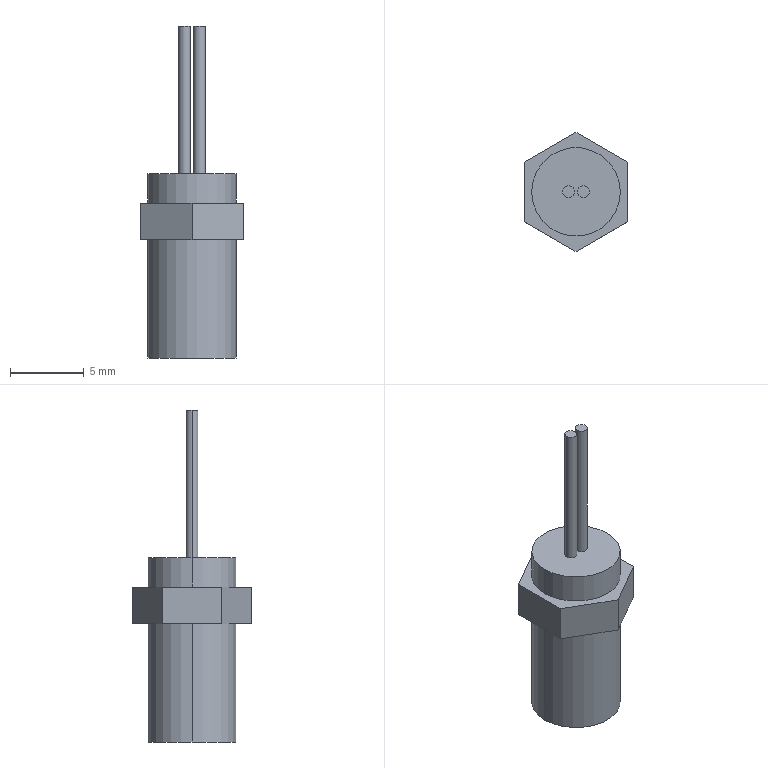Part | SolidWorks | features ICE 3, Extrusion 1 | 1 solid | 20 faces | box 7 x 8.083 x 22.5 mm | volume 398.885 mm3 | plane 12 | cylinder 8 | commonest cylinder face diameters 0.8 x4 6 x4
STEP:
#1=CARTESIAN_POINT('',(-0.1,0.,22.5));
#2=VERTEX_POINT('',#1);
#3=CARTESIAN_POINT('',(-0.9,0.,22.5));
#4=VERTEX_POINT('',#3);
#5=CARTESIAN_POINT('',(-0.5,0.,22.5));
#6=DIRECTION('',(0.,0.,1.));
#7=DIRECTION('',(1.,0.,0.));
#8=AXIS2_PLACEMENT_3D('',#5,#6,#7);
#9=CIRCLE('',#8,0.4);
#10=EDGE_CURVE('',#2,#4,#9,.T.);
#11=ORIENTED_EDGE('',*,*,#10,.F.);
#12=CARTESIAN_POINT('',(-0.1,0.,12.5));
#13=VERTEX_POINT('',#12);
#14=CARTESIAN_POINT('',(-0.1,0.,22.5));
#15=DIRECTION('',(0.,0.,-1.));
#16=VECTOR('',#15,1000.);
#17=LINE('',#14,#16);
#18=EDGE_CURVE('',#2,#13,#17,.T.);
#19=ORIENTED_EDGE('',*,*,#18,.T.);
#20=CARTESIAN_POINT('',(-0.9,0.,12.5));
#21=VERTEX_POINT('',#20);
#22=CARTESIAN_POINT('',(-0.5,0.,12.5));
#23=DIRECTION('',(0.,0.,1.));
#24=DIRECTION('',(1.,0.,0.));
#25=AXIS2_PLACEMENT_3D('',#22,#23,#24);
#26=CIRCLE('',#25,0.4);
#27=EDGE_CURVE('',#13,#21,#26,.T.);
#28=ORIENTED_EDGE('',*,*,#27,.T.);
#29=CARTESIAN_POINT('',(-0.9,0.,22.5));
#30=DIRECTION('',(0.,0.,-1.));
#31=VECTOR('',#30,1000.);
#32=LINE('',#29,#31);
#33=EDGE_CURVE('',#4,#21,#32,.T.);
#34=ORIENTED_EDGE('',*,*,#33,.F.);
#35=EDGE_LOOP('',(#11,#19,#28,#34));
#36=FACE_OUTER_BOUND('',#35,.T.);
#37=CARTESIAN_POINT('',(-0.5,0.,22.5));
#38=DIRECTION('',(0.,0.,-1.));
#39=DIRECTION('',(-1.,0.,0.));
#40=AXIS2_PLACEMENT_3D('',#37,#38,#39);
#41=CYLINDRICAL_SURFACE('',#40,0.4);
#42=ADVANCED_FACE('',(#36),#41,.T.);
#43=CARTESIAN_POINT('',(0.9,0.,22.5));
#44=VERTEX_POINT('',#43);
#45=CARTESIAN_POINT('',(0.1,0.,22.5));
#46=VERTEX_POINT('',#45);
#47=CARTESIAN_POINT('',(0.5,0.,22.5));
#48=DIRECTION('',(0.,0.,1.));
#49=DIRECTION('',(1.,0.,0.));
#50=AXIS2_PLACEMENT_3D('',#47,#48,#49);
#51=CIRCLE('',#50,0.4);
#52=EDGE_CURVE('',#44,#46,#51,.T.);
#53=ORIENTED_EDGE('',*,*,#52,.F.);
#54=CARTESIAN_POINT('',(0.9,0.,12.5));
#55=VERTEX_POINT('',#54);
#56=CARTESIAN_POINT('',(0.9,0.,22.5));
#57=DIRECTION('',(0.,0.,-1.));
#58=VECTOR('',#57,1000.);
#59=LINE('',#56,#58);
#60=EDGE_CURVE('',#44,#55,#59,.T.);
#61=ORIENTED_EDGE('',*,*,#60,.T.);
#62=CARTESIAN_POINT('',(0.1,0.,12.5));
#63=VERTEX_POINT('',#62);
#64=CARTESIAN_POINT('',(0.5,0.,12.5));
#65=DIRECTION('',(0.,0.,1.));
#66=DIRECTION('',(1.,0.,0.));
#67=AXIS2_PLACEMENT_3D('',#64,#65,#66);
#68=CIRCLE('',#67,0.4);
#69=EDGE_CURVE('',#55,#63,#68,.T.);
#70=ORIENTED_EDGE('',*,*,#69,.T.);
#71=CARTESIAN_POINT('',(0.1,0.,22.5));
#72=DIRECTION('',(0.,0.,-1.));
#73=VECTOR('',#72,1000.);
#74=LINE('',#71,#73);
#75=EDGE_CURVE('',#46,#63,#74,.T.);
#76=ORIENTED_EDGE('',*,*,#75,.F.);
#77=EDGE_LOOP('',(#53,#61,#70,#76));
#78=FACE_OUTER_BOUND('',#77,.T.);
#79=CARTESIAN_POINT('',(0.5,0.,22.5));
#80=DIRECTION('',(0.,0.,-1.));
#81=DIRECTION('',(-1.,0.,0.));
#82=AXIS2_PLACEMENT_3D('',#79,#80,#81);
#83=CYLINDRICAL_SURFACE('',#82,0.4);
#84=ADVANCED_FACE('',(#78),#83,.T.);
#85=CARTESIAN_POINT('',(3.,0.,12.5));
#86=VERTEX_POINT('',#85);
#87=CARTESIAN_POINT('',(-3.,0.,12.5));
#88=VERTEX_POINT('',#87);
#89=CARTESIAN_POINT('',(0.,0.,12.5));
#90=DIRECTION('',(0.,0.,1.));
#91=DIRECTION('',(1.,0.,0.));
#92=AXIS2_PLACEMENT_3D('',#89,#90,#91);
#93=CIRCLE('',#92,3.);
#94=EDGE_CURVE('',#86,#88,#93,.T.);
#95=ORIENTED_EDGE('',*,*,#94,.F.);
#96=CARTESIAN_POINT('',(3.,0.,10.5));
#97=VERTEX_POINT('',#96);
#98=CARTESIAN_POINT('',(3.,0.,12.5));
#99=DIRECTION('',(0.,0.,-1.));
#100=VECTOR('',#99,1000.);
#101=LINE('',#98,#100);
#102=EDGE_CURVE('',#86,#97,#101,.T.);
#103=ORIENTED_EDGE('',*,*,#102,.T.);
#104=CARTESIAN_POINT('',(-3.,0.,10.5));
#105=VERTEX_POINT('',#104);
#106=CARTESIAN_POINT('',(0.,0.,10.5));
#107=DIRECTION('',(0.,0.,1.));
#108=DIRECTION('',(1.,0.,0.));
#109=AXIS2_PLACEMENT_3D('',#106,#107,#108);
#110=CIRCLE('',#109,3.);
#111=EDGE_CURVE('',#97,#105,#110,.T.);
#112=ORIENTED_EDGE('',*,*,#111,.T.);
#113=CARTESIAN_POINT('',(-3.,0.,12.5));
#114=DIRECTION('',(0.,0.,-1.));
#115=VECTOR('',#114,1000.);
#116=LINE('',#113,#115);
#117=EDGE_CURVE('',#88,#105,#116,.T.);
#118=ORIENTED_EDGE('',*,*,#117,.F.);
#119=EDGE_LOOP('',(#95,#103,#112,#118));
#120=FACE_OUTER_BOUND('',#119,.T.);
#121=CARTESIAN_POINT('',(0.,0.,12.5));
#122=DIRECTION('',(0.,0.,-1.));
#123=DIRECTION('',(-1.,0.,0.));
#124=AXIS2_PLACEMENT_3D('',#121,#122,#123);
#125=CYLINDRICAL_SURFACE('',#124,3.);
#126=ADVANCED_FACE('',(#120),#125,.T.);
#127=CARTESIAN_POINT('',(3.,0.,8.));
#128=VERTEX_POINT('',#127);
#129=CARTESIAN_POINT('',(-3.,0.,8.));
#130=VERTEX_POINT('',#129);
#131=CARTESIAN_POINT('',(0.,0.,8.));
#132=DIRECTION('',(0.,0.,1.));
#133=DIRECTION('',(1.,0.,0.));
#134=AXIS2_PLACEMENT_3D('',#131,#132,#133);
#135=CIRCLE('',#134,3.);
#136=EDGE_CURVE('',#128,#130,#135,.T.);
#137=ORIENTED_EDGE('',*,*,#136,.F.);
#138=CARTESIAN_POINT('',(3.,0.,0.));
#139=VERTEX_POINT('',#138);
#140=CARTESIAN_POINT('',(3.,0.,8.));
#141=DIRECTION('',(0.,0.,-1.));
#142=VECTOR('',#141,1000.);
#143=LINE('',#140,#142);
#144=EDGE_CURVE('',#128,#139,#143,.T.);
#145=ORIENTED_EDGE('',*,*,#144,.T.);
#146=CARTESIAN_POINT('',(-3.,0.,0.));
#147=VERTEX_POINT('',#146);
#148=CARTESIAN_POINT('',(0.,0.,0.));
#149=DIRECTION('',(0.,0.,1.));
#150=DIRECTION('',(1.,0.,0.));
#151=AXIS2_PLACEMENT_3D('',#148,#149,#150);
#152=CIRCLE('',#151,3.);
#153=EDGE_CURVE('',#139,#147,#152,.T.);
#154=ORIENTED_EDGE('',*,*,#153,.T.);
#155=CARTESIAN_POINT('',(-3.,0.,8.));
#156=DIRECTION('',(0.,0.,-1.));
#157=VECTOR('',#156,1000.);
#158=LINE('',#155,#157);
#159=EDGE_CURVE('',#130,#147,#158,.T.);
#160=ORIENTED_EDGE('',*,*,#159,.F.);
#161=EDGE_LOOP('',(#137,#145,#154,#160));
#162=FACE_OUTER_BOUND('',#161,.T.);
#163=CARTESIAN_POINT('',(0.,0.,8.));
#164=DIRECTION('',(0.,0.,-1.));
#165=DIRECTION('',(-1.,0.,0.));
#166=AXIS2_PLACEMENT_3D('',#163,#164,#165);
#167=CYLINDRICAL_SURFACE('',#166,3.);
#168=ADVANCED_FACE('',(#162),#167,.T.);
#169=CARTESIAN_POINT('',(0.5,0.,12.5));
#170=DIRECTION('',(0.,0.,1.));
#171=DIRECTION('',(1.,0.,0.));
#172=AXIS2_PLACEMENT_3D('',#169,#170,#171);
#173=CIRCLE('',#172,0.4);
#174=EDGE_CURVE('',#63,#55,#173,.T.);
#175=ORIENTED_EDGE('',*,*,#174,.F.);
#176=ORIENTED_EDGE('',*,*,#69,.F.);
#177=EDGE_LOOP('',(#175,#176));
#178=FACE_BOUND('',#177,.T.);
#179=CARTESIAN_POINT('',(0.,0.,12.5));
#180=DIRECTION('',(0.,0.,1.));
#181=DIRECTION('',(1.,0.,0.));
#182=AXIS2_PLACEMENT_3D('',#179,#180,#181);
#183=CIRCLE('',#182,3.);
#184=EDGE_CURVE('',#88,#86,#183,.T.);
#185=ORIENTED_EDGE('',*,*,#184,.T.);
#186=ORIENTED_EDGE('',*,*,#94,.T.);
#187=EDGE_LOOP('',(#185,#186));
#188=FACE_OUTER_BOUND('',#187,.T.);
#189=CARTESIAN_POINT('',(-0.5,0.,12.5));
#190=DIRECTION('',(0.,0.,1.));
#191=DIRECTION('',(1.,0.,0.));
#192=AXIS2_PLACEMENT_3D('',#189,#190,#191);
#193=CIRCLE('',#192,0.4);
#194=EDGE_CURVE('',#21,#13,#193,.T.);
#195=ORIENTED_EDGE('',*,*,#194,.F.);
#196=ORIENTED_EDGE('',*,*,#27,.F.);
#197=EDGE_LOOP('',(#195,#196));
#198=FACE_BOUND('',#197,.T.);
#199=CARTESIAN_POINT('',(0.,0.,12.5));
#200=DIRECTION('',(0.,0.,1.));
#201=DIRECTION('',(1.,0.,0.));
#202=AXIS2_PLACEMENT_3D('',#199,#200,#201);
#203=PLANE('',#202);
#204=ADVANCED_FACE('',(#178,#188,#198),#203,.T.);
#205=CARTESIAN_POINT('',(3.5,2.021,10.5));
#206=VERTEX_POINT('',#205);
#207=CARTESIAN_POINT('',(0.,4.041,10.5));
#208=VERTEX_POINT('',#207);
#209=CARTESIAN_POINT('',(3.5,2.021,10.5));
#210=DIRECTION('',(-0.866,0.5,0.));
#211=VECTOR('',#210,1000.);
#212=LINE('',#209,#211);
#213=EDGE_CURVE('',#206,#208,#212,.T.);
#214=ORIENTED_EDGE('',*,*,#213,.T.);
#215=CARTESIAN_POINT('',(-3.5,2.021,10.5));
#216=VERTEX_POINT('',#215);
#217=CARTESIAN_POINT('',(0.,4.041,10.5));
#218=DIRECTION('',(-0.866,-0.5,0.));
#219=VECTOR('',#218,1000.);
#220=LINE('',#217,#219);
#221=EDGE_CURVE('',#208,#216,#220,.T.);
#222=ORIENTED_EDGE('',*,*,#221,.T.);
#223=CARTESIAN_POINT('',(-3.5,-2.021,10.5));
#224=VERTEX_POINT('',#223);
#225=CARTESIAN_POINT('',(-3.5,2.021,10.5));
#226=DIRECTION('',(0.,-1.,0.));
#227=VECTOR('',#226,1000.);
#228=LINE('',#225,#227);
#229=EDGE_CURVE('',#216,#224,#228,.T.);
#230=ORIENTED_EDGE('',*,*,#229,.T.);
#231=CARTESIAN_POINT('',(0.,-4.041,10.5));
#232=VERTEX_POINT('',#231);
#233=CARTESIAN_POINT('',(-3.5,-2.021,10.5));
#234=DIRECTION('',(0.866,-0.5,0.));
#235=VECTOR('',#234,1000.);
#236=LINE('',#233,#235);
#237=EDGE_CURVE('',#224,#232,#236,.T.);
#238=ORIENTED_EDGE('',*,*,#237,.T.);
#239=CARTESIAN_POINT('',(3.5,-2.021,10.5));
#240=VERTEX_POINT('',#239);
#241=CARTESIAN_POINT('',(0.,-4.041,10.5));
#242=DIRECTION('',(0.866,0.5,0.));
#243=VECTOR('',#242,1000.);
#244=LINE('',#241,#243);
#245=EDGE_CURVE('',#232,#240,#244,.T.);
#246=ORIENTED_EDGE('',*,*,#245,.T.);
#247=CARTESIAN_POINT('',(3.5,-2.021,10.5));
#248=DIRECTION('',(0.,1.,0.));
#249=VECTOR('',#248,1000.);
#250=LINE('',#247,#249);
#251=EDGE_CURVE('',#240,#206,#250,.T.);
#252=ORIENTED_EDGE('',*,*,#251,.T.);
#253=EDGE_LOOP('',(#214,#222,#230,#238,#246,#252));
#254=FACE_OUTER_BOUND('',#253,.T.);
#255=CARTESIAN_POINT('',(0.,0.,10.5));
#256=DIRECTION('',(0.,0.,1.));
#257=DIRECTION('',(1.,0.,0.));
#258=AXIS2_PLACEMENT_3D('',#255,#256,#257);
#259=CIRCLE('',#258,3.);
#260=EDGE_CURVE('',#105,#97,#259,.T.);
#261=ORIENTED_EDGE('',*,*,#260,.F.);
#262=ORIENTED_EDGE('',*,*,#111,.F.);
#263=EDGE_LOOP('',(#261,#262));
#264=FACE_BOUND('',#263,.T.);
#265=CARTESIAN_POINT('',(0.,0.,10.5));
#266=DIRECTION('',(0.,0.,1.));
#267=DIRECTION('',(1.,0.,0.));
#268=AXIS2_PLACEMENT_3D('',#265,#266,#267);
#269=PLANE('',#268);
#270=ADVANCED_FACE('',(#254,#264),#269,.T.);
#271=ORIENTED_EDGE('',*,*,#144,.F.);
#272=CARTESIAN_POINT('',(0.,0.,8.));
#273=DIRECTION('',(0.,0.,1.));
#274=DIRECTION('',(1.,0.,0.));
#275=AXIS2_PLACEMENT_3D('',#272,#273,#274);
#276=CIRCLE('',#275,3.);
#277=EDGE_CURVE('',#130,#128,#276,.T.);
#278=ORIENTED_EDGE('',*,*,#277,.F.);
#279=ORIENTED_EDGE('',*,*,#159,.T.);
#280=CARTESIAN_POINT('',(0.,0.,0.));
#281=DIRECTION('',(0.,0.,1.));
#282=DIRECTION('',(1.,0.,0.));
#283=AXIS2_PLACEMENT_3D('',#280,#281,#282);
#284=CIRCLE('',#283,3.);
#285=EDGE_CURVE('',#147,#139,#284,.T.);
#286=ORIENTED_EDGE('',*,*,#285,.T.);
#287=EDGE_LOOP('',(#271,#278,#279,#286));
#288=FACE_OUTER_BOUND('',#287,.T.);
#289=CARTESIAN_POINT('',(0.,0.,8.));
#290=DIRECTION('',(0.,0.,-1.));
#291=DIRECTION('',(-1.,0.,0.));
#292=AXIS2_PLACEMENT_3D('',#289,#290,#291);
#293=CYLINDRICAL_SURFACE('',#292,3.);
#294=ADVANCED_FACE('',(#288),#293,.T.);
#295=ORIENTED_EDGE('',*,*,#285,.F.);
#296=ORIENTED_EDGE('',*,*,#153,.F.);
#297=EDGE_LOOP('',(#295,#296));
#298=FACE_OUTER_BOUND('',#297,.T.);
#299=CARTESIAN_POINT('',(0.,0.,0.));
#300=DIRECTION('',(0.,0.,1.));
#301=DIRECTION('',(1.,0.,0.));
#302=AXIS2_PLACEMENT_3D('',#299,#300,#301);
#303=PLANE('',#302);
#304=ADVANCED_FACE('',(#298),#303,.F.);
#305=CARTESIAN_POINT('',(3.5,2.021,8.));
#306=VERTEX_POINT('',#305);
#307=CARTESIAN_POINT('',(0.,4.041,8.));
#308=VERTEX_POINT('',#307);
#309=CARTESIAN_POINT('',(3.5,2.021,8.));
#310=DIRECTION('',(-0.866,0.5,0.));
#311=VECTOR('',#310,1000.);
#312=LINE('',#309,#311);
#313=EDGE_CURVE('',#306,#308,#312,.T.);
#314=ORIENTED_EDGE('',*,*,#313,.F.);
#315=CARTESIAN_POINT('',(3.5,-2.021,8.));
#316=VERTEX_POINT('',#315);
#317=CARTESIAN_POINT('',(3.5,-2.021,8.));
#318=DIRECTION('',(0.,1.,0.));
#319=VECTOR('',#318,1000.);
#320=LINE('',#317,#319);
#321=EDGE_CURVE('',#316,#306,#320,.T.);
#322=ORIENTED_EDGE('',*,*,#321,.F.);
#323=CARTESIAN_POINT('',(0.,-4.041,8.));
#324=VERTEX_POINT('',#323);
#325=CARTESIAN_POINT('',(0.,-4.041,8.));
#326=DIRECTION('',(0.866,0.5,0.));
#327=VECTOR('',#326,1000.);
#328=LINE('',#325,#327);
#329=EDGE_CURVE('',#324,#316,#328,.T.);
#330=ORIENTED_EDGE('',*,*,#329,.F.);
#331=CARTESIAN_POINT('',(-3.5,-2.021,8.));
#332=VERTEX_POINT('',#331);
#333=CARTESIAN_POINT('',(-3.5,-2.021,8.));
#334=DIRECTION('',(0.866,-0.5,0.));
#335=VECTOR('',#334,1000.);
#336=LINE('',#333,#335);
#337=EDGE_CURVE('',#332,#324,#336,.T.);
#338=ORIENTED_EDGE('',*,*,#337,.F.);
#339=CARTESIAN_POINT('',(-3.5,2.021,8.));
#340=VERTEX_POINT('',#339);
#341=CARTESIAN_POINT('',(-3.5,2.021,8.));
#342=DIRECTION('',(0.,-1.,0.));
#343=VECTOR('',#342,1000.);
#344=LINE('',#341,#343);
#345=EDGE_CURVE('',#340,#332,#344,.T.);
#346=ORIENTED_EDGE('',*,*,#345,.F.);
#347=CARTESIAN_POINT('',(0.,4.041,8.));
#348=DIRECTION('',(-0.866,-0.5,0.));
#349=VECTOR('',#348,1000.);
#350=LINE('',#347,#349);
#351=EDGE_CURVE('',#308,#340,#350,.T.);
#352=ORIENTED_EDGE('',*,*,#351,.F.);
#353=EDGE_LOOP('',(#314,#322,#330,#338,#346,#352));
#354=FACE_OUTER_BOUND('',#353,.T.);
#355=ORIENTED_EDGE('',*,*,#277,.T.);
#356=ORIENTED_EDGE('',*,*,#136,.T.);
#357=EDGE_LOOP('',(#355,#356));
#358=FACE_BOUND('',#357,.T.);
#359=CARTESIAN_POINT('',(0.,0.,8.));
#360=DIRECTION('',(0.,0.,1.));
#361=DIRECTION('',(1.,0.,0.));
#362=AXIS2_PLACEMENT_3D('',#359,#360,#361);
#363=PLANE('',#362);
#364=ADVANCED_FACE('',(#354,#358),#363,.F.);
#365=ORIENTED_EDGE('',*,*,#313,.T.);
#366=CARTESIAN_POINT('',(0.,4.041,10.5));
#367=DIRECTION('',(0.,0.,-1.));
#368=VECTOR('',#367,1000.);
#369=LINE('',#366,#368);
#370=EDGE_CURVE('',#208,#308,#369,.T.);
#371=ORIENTED_EDGE('',*,*,#370,.F.);
#372=ORIENTED_EDGE('',*,*,#213,.F.);
#373=CARTESIAN_POINT('',(3.5,2.021,10.5));
#374=DIRECTION('',(0.,0.,-1.));
#375=VECTOR('',#374,1000.);
#376=LINE('',#373,#375);
#377=EDGE_CURVE('',#206,#306,#376,.T.);
#378=ORIENTED_EDGE('',*,*,#377,.T.);
#379=EDGE_LOOP('',(#365,#371,#372,#378));
#380=FACE_OUTER_BOUND('',#379,.T.);
#381=CARTESIAN_POINT('',(3.5,2.021,10.5));
#382=DIRECTION('',(-0.5,-0.866,0.));
#383=DIRECTION('',(0.866,-0.5,0.));
#384=AXIS2_PLACEMENT_3D('',#381,#382,#383);
#385=PLANE('',#384);
#386=ADVANCED_FACE('',(#380),#385,.F.);
#387=ORIENTED_EDGE('',*,*,#351,.T.);
#388=CARTESIAN_POINT('',(-3.5,2.021,10.5));
#389=DIRECTION('',(0.,0.,-1.));
#390=VECTOR('',#389,1000.);
#391=LINE('',#388,#390);
#392=EDGE_CURVE('',#216,#340,#391,.T.);
#393=ORIENTED_EDGE('',*,*,#392,.F.);
#394=ORIENTED_EDGE('',*,*,#221,.F.);
#395=ORIENTED_EDGE('',*,*,#370,.T.);
#396=EDGE_LOOP('',(#387,#393,#394,#395));
#397=FACE_OUTER_BOUND('',#396,.T.);
#398=CARTESIAN_POINT('',(0.,4.041,10.5));
#399=DIRECTION('',(0.5,-0.866,0.));
#400=DIRECTION('',(0.866,0.5,0.));
#401=AXIS2_PLACEMENT_3D('',#398,#399,#400);
#402=PLANE('',#401);
#403=ADVANCED_FACE('',(#397),#402,.F.);
#404=ORIENTED_EDGE('',*,*,#345,.T.);
#405=CARTESIAN_POINT('',(-3.5,-2.021,10.5));
#406=DIRECTION('',(0.,0.,-1.));
#407=VECTOR('',#406,1000.);
#408=LINE('',#405,#407);
#409=EDGE_CURVE('',#224,#332,#408,.T.);
#410=ORIENTED_EDGE('',*,*,#409,.F.);
#411=ORIENTED_EDGE('',*,*,#229,.F.);
#412=ORIENTED_EDGE('',*,*,#392,.T.);
#413=EDGE_LOOP('',(#404,#410,#411,#412));
#414=FACE_OUTER_BOUND('',#413,.T.);
#415=CARTESIAN_POINT('',(-3.5,2.021,10.5));
#416=DIRECTION('',(1.,0.,0.));
#417=DIRECTION('',(0.,1.,0.));
#418=AXIS2_PLACEMENT_3D('',#415,#416,#417);
#419=PLANE('',#418);
#420=ADVANCED_FACE('',(#414),#419,.F.);
#421=ORIENTED_EDGE('',*,*,#337,.T.);
#422=CARTESIAN_POINT('',(0.,-4.041,10.5));
#423=DIRECTION('',(0.,0.,-1.));
#424=VECTOR('',#423,1000.);
#425=LINE('',#422,#424);
#426=EDGE_CURVE('',#232,#324,#425,.T.);
#427=ORIENTED_EDGE('',*,*,#426,.F.);
#428=ORIENTED_EDGE('',*,*,#237,.F.);
#429=ORIENTED_EDGE('',*,*,#409,.T.);
#430=EDGE_LOOP('',(#421,#427,#428,#429));
#431=FACE_OUTER_BOUND('',#430,.T.);
#432=CARTESIAN_POINT('',(-3.5,-2.021,10.5));
#433=DIRECTION('',(0.5,0.866,0.));
#434=DIRECTION('',(-0.866,0.5,0.));
#435=AXIS2_PLACEMENT_3D('',#432,#433,#434);
#436=PLANE('',#435);
#437=ADVANCED_FACE('',(#431),#436,.F.);
#438=ORIENTED_EDGE('',*,*,#329,.T.);
#439=CARTESIAN_POINT('',(3.5,-2.021,10.5));
#440=DIRECTION('',(0.,0.,-1.));
#441=VECTOR('',#440,1000.);
#442=LINE('',#439,#441);
#443=EDGE_CURVE('',#240,#316,#442,.T.);
#444=ORIENTED_EDGE('',*,*,#443,.F.);
#445=ORIENTED_EDGE('',*,*,#245,.F.);
#446=ORIENTED_EDGE('',*,*,#426,.T.);
#447=EDGE_LOOP('',(#438,#444,#445,#446));
#448=FACE_OUTER_BOUND('',#447,.T.);
#449=CARTESIAN_POINT('',(0.,-4.041,10.5));
#450=DIRECTION('',(-0.5,0.866,0.));
#451=DIRECTION('',(-0.866,-0.5,0.));
#452=AXIS2_PLACEMENT_3D('',#449,#450,#451);
#453=PLANE('',#452);
#454=ADVANCED_FACE('',(#448),#453,.F.);
#455=ORIENTED_EDGE('',*,*,#321,.T.);
#456=ORIENTED_EDGE('',*,*,#377,.F.);
#457=ORIENTED_EDGE('',*,*,#251,.F.);
#458=ORIENTED_EDGE('',*,*,#443,.T.);
#459=EDGE_LOOP('',(#455,#456,#457,#458));
#460=FACE_OUTER_BOUND('',#459,.T.);
#461=CARTESIAN_POINT('',(3.5,-2.021,10.5));
#462=DIRECTION('',(-1.,0.,0.));
#463=DIRECTION('',(0.,-1.,0.));
#464=AXIS2_PLACEMENT_3D('',#461,#462,#463);
#465=PLANE('',#464);
#466=ADVANCED_FACE('',(#460),#465,.F.);
#467=ORIENTED_EDGE('',*,*,#102,.F.);
#468=ORIENTED_EDGE('',*,*,#184,.F.);
#469=ORIENTED_EDGE('',*,*,#117,.T.);
#470=ORIENTED_EDGE('',*,*,#260,.T.);
#471=EDGE_LOOP('',(#467,#468,#469,#470));
#472=FACE_OUTER_BOUND('',#471,.T.);
#473=CARTESIAN_POINT('',(0.,0.,12.5));
#474=DIRECTION('',(0.,0.,-1.));
#475=DIRECTION('',(-1.,0.,0.));
#476=AXIS2_PLACEMENT_3D('',#473,#474,#475);
#477=CYLINDRICAL_SURFACE('',#476,3.);
#478=ADVANCED_FACE('',(#472),#477,.T.);
#479=ORIENTED_EDGE('',*,*,#60,.F.);
#480=CARTESIAN_POINT('',(0.5,0.,22.5));
#481=DIRECTION('',(0.,0.,1.));
#482=DIRECTION('',(1.,0.,0.));
#483=AXIS2_PLACEMENT_3D('',#480,#481,#482);
#484=CIRCLE('',#483,0.4);
#485=EDGE_CURVE('',#46,#44,#484,.T.);
#486=ORIENTED_EDGE('',*,*,#485,.F.);
#487=ORIENTED_EDGE('',*,*,#75,.T.);
#488=ORIENTED_EDGE('',*,*,#174,.T.);
#489=EDGE_LOOP('',(#479,#486,#487,#488));
#490=FACE_OUTER_BOUND('',#489,.T.);
#491=CARTESIAN_POINT('',(0.5,0.,22.5));
#492=DIRECTION('',(0.,0.,-1.));
#493=DIRECTION('',(-1.,0.,0.));
#494=AXIS2_PLACEMENT_3D('',#491,#492,#493);
#495=CYLINDRICAL_SURFACE('',#494,0.4);
#496=ADVANCED_FACE('',(#490),#495,.T.);
#497=ORIENTED_EDGE('',*,*,#485,.T.);
#498=ORIENTED_EDGE('',*,*,#52,.T.);
#499=EDGE_LOOP('',(#497,#498));
#500=FACE_OUTER_BOUND('',#499,.T.);
#501=CARTESIAN_POINT('',(0.5,0.,22.5));
#502=DIRECTION('',(0.,0.,1.));
#503=DIRECTION('',(1.,0.,0.));
#504=AXIS2_PLACEMENT_3D('',#501,#502,#503);
#505=PLANE('',#504);
#506=ADVANCED_FACE('',(#500),#505,.T.);
#507=ORIENTED_EDGE('',*,*,#18,.F.);
#508=CARTESIAN_POINT('',(-0.5,0.,22.5));
#509=DIRECTION('',(0.,0.,1.));
#510=DIRECTION('',(1.,0.,0.));
#511=AXIS2_PLACEMENT_3D('',#508,#509,#510);
#512=CIRCLE('',#511,0.4);
#513=EDGE_CURVE('',#4,#2,#512,.T.);
#514=ORIENTED_EDGE('',*,*,#513,.F.);
#515=ORIENTED_EDGE('',*,*,#33,.T.);
#516=ORIENTED_EDGE('',*,*,#194,.T.);
#517=EDGE_LOOP('',(#507,#514,#515,#516));
#518=FACE_OUTER_BOUND('',#517,.T.);
#519=CARTESIAN_POINT('',(-0.5,0.,22.5));
#520=DIRECTION('',(0.,0.,-1.));
#521=DIRECTION('',(-1.,0.,0.));
#522=AXIS2_PLACEMENT_3D('',#519,#520,#521);
#523=CYLINDRICAL_SURFACE('',#522,0.4);
#524=ADVANCED_FACE('',(#518),#523,.T.);
#525=ORIENTED_EDGE('',*,*,#513,.T.);
#526=ORIENTED_EDGE('',*,*,#10,.T.);
#527=EDGE_LOOP('',(#525,#526));
#528=FACE_OUTER_BOUND('',#527,.T.);
#529=CARTESIAN_POINT('',(-0.5,0.,22.5));
#530=DIRECTION('',(0.,0.,1.));
#531=DIRECTION('',(1.,0.,0.));
#532=AXIS2_PLACEMENT_3D('',#529,#530,#531);
#533=PLANE('',#532);
#534=ADVANCED_FACE('',(#528),#533,.T.);
#535=CLOSED_SHELL('',(#42,#84,#126,#168,#204,#270,#294,#304,#364,#386,#403,#420,#437,#454,#466,#478,#496,#506,#524,#534));
#536=MANIFOLD_SOLID_BREP('',#535);
#537=CARTESIAN_POINT('',(0.,0.,0.));
#538=DIRECTION('',(0.,0.,1.));
#539=DIRECTION('',(1.,0.,0.));
#540=AXIS2_PLACEMENT_3D('',#537,#538,#539);
#541=(LENGTH_UNIT()NAMED_UNIT(*)SI_UNIT(.MILLI.,.METRE.));
#542=UNCERTAINTY_MEASURE_WITH_UNIT(LENGTH_MEASURE(0.00001),#541,'','');
#543=(NAMED_UNIT(*)PLANE_ANGLE_UNIT()SI_UNIT($,.RADIAN.));
#544=(NAMED_UNIT(*)SI_UNIT($,.STERADIAN.)SOLID_ANGLE_UNIT());
#545=(GEOMETRIC_REPRESENTATION_CONTEXT(3)GLOBAL_UNCERTAINTY_ASSIGNED_CONTEXT((#542))GLOBAL_UNIT_ASSIGNED_CONTEXT((#541,#543,#544))REPRESENTATION_CONTEXT('',''));
#546=ADVANCED_BREP_SHAPE_REPRESENTATION('',(#536,#540),#545);